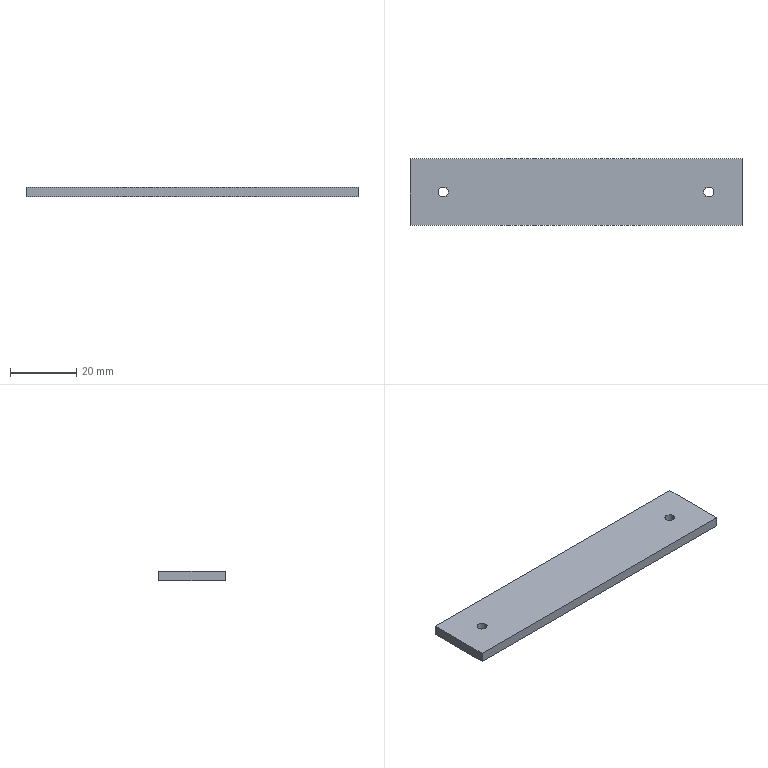Part | SolidWorks | features BaseBody 1 | 1 solid | 10 faces | box 100 x 20 x 3 mm | volume 5958 mm3 | plane 6 | cylinder 4 | commonest cylinder face diameters 3 x4
STEP:
#1=CARTESIAN_POINT('',(38.5,0.,0.));
#2=VERTEX_POINT('',#1);
#3=CARTESIAN_POINT('',(41.5,0.,0.));
#4=VERTEX_POINT('',#3);
#5=CARTESIAN_POINT('',(40.,0.,0.));
#6=DIRECTION('',(0.,0.,1.));
#7=DIRECTION('',(1.,0.,0.));
#8=AXIS2_PLACEMENT_3D('',#5,#6,#7);
#9=CIRCLE('',#8,1.5);
#10=EDGE_CURVE('',#2,#4,#9,.T.);
#11=ORIENTED_EDGE('',*,*,#10,.F.);
#12=CARTESIAN_POINT('',(38.5,0.,3.));
#13=VERTEX_POINT('',#12);
#14=CARTESIAN_POINT('',(38.5,0.,0.));
#15=DIRECTION('',(0.,0.,1.));
#16=VECTOR('',#15,1000.);
#17=LINE('',#14,#16);
#18=EDGE_CURVE('',#2,#13,#17,.T.);
#19=ORIENTED_EDGE('',*,*,#18,.T.);
#20=CARTESIAN_POINT('',(41.5,0.,3.));
#21=VERTEX_POINT('',#20);
#22=CARTESIAN_POINT('',(40.,0.,3.));
#23=DIRECTION('',(0.,0.,-1.));
#24=DIRECTION('',(1.,0.,0.));
#25=AXIS2_PLACEMENT_3D('',#22,#23,#24);
#26=CIRCLE('',#25,1.5);
#27=EDGE_CURVE('',#21,#13,#26,.T.);
#28=ORIENTED_EDGE('',*,*,#27,.F.);
#29=CARTESIAN_POINT('',(41.5,0.,0.));
#30=DIRECTION('',(0.,0.,1.));
#31=VECTOR('',#30,1000.);
#32=LINE('',#29,#31);
#33=EDGE_CURVE('',#4,#21,#32,.T.);
#34=ORIENTED_EDGE('',*,*,#33,.F.);
#35=EDGE_LOOP('',(#11,#19,#28,#34));
#36=FACE_OUTER_BOUND('',#35,.T.);
#37=CARTESIAN_POINT('',(40.,0.,0.));
#38=DIRECTION('',(0.,0.,1.));
#39=DIRECTION('',(1.,0.,0.));
#40=AXIS2_PLACEMENT_3D('',#37,#38,#39);
#41=CYLINDRICAL_SURFACE('',#40,1.5);
#42=ADVANCED_FACE('',(#36),#41,.F.);
#43=CARTESIAN_POINT('',(-41.5,0.,0.));
#44=VERTEX_POINT('',#43);
#45=CARTESIAN_POINT('',(-38.5,0.,0.));
#46=VERTEX_POINT('',#45);
#47=CARTESIAN_POINT('',(-40.,0.,0.));
#48=DIRECTION('',(0.,0.,1.));
#49=DIRECTION('',(1.,0.,0.));
#50=AXIS2_PLACEMENT_3D('',#47,#48,#49);
#51=CIRCLE('',#50,1.5);
#52=EDGE_CURVE('',#44,#46,#51,.T.);
#53=ORIENTED_EDGE('',*,*,#52,.F.);
#54=CARTESIAN_POINT('',(-41.5,0.,3.));
#55=VERTEX_POINT('',#54);
#56=CARTESIAN_POINT('',(-41.5,0.,0.));
#57=DIRECTION('',(0.,0.,1.));
#58=VECTOR('',#57,1000.);
#59=LINE('',#56,#58);
#60=EDGE_CURVE('',#44,#55,#59,.T.);
#61=ORIENTED_EDGE('',*,*,#60,.T.);
#62=CARTESIAN_POINT('',(-38.5,0.,3.));
#63=VERTEX_POINT('',#62);
#64=CARTESIAN_POINT('',(-40.,0.,3.));
#65=DIRECTION('',(0.,0.,-1.));
#66=DIRECTION('',(1.,0.,0.));
#67=AXIS2_PLACEMENT_3D('',#64,#65,#66);
#68=CIRCLE('',#67,1.5);
#69=EDGE_CURVE('',#63,#55,#68,.T.);
#70=ORIENTED_EDGE('',*,*,#69,.F.);
#71=CARTESIAN_POINT('',(-38.5,0.,0.));
#72=DIRECTION('',(0.,0.,1.));
#73=VECTOR('',#72,1000.);
#74=LINE('',#71,#73);
#75=EDGE_CURVE('',#46,#63,#74,.T.);
#76=ORIENTED_EDGE('',*,*,#75,.F.);
#77=EDGE_LOOP('',(#53,#61,#70,#76));
#78=FACE_OUTER_BOUND('',#77,.T.);
#79=CARTESIAN_POINT('',(-40.,0.,0.));
#80=DIRECTION('',(0.,0.,1.));
#81=DIRECTION('',(1.,0.,0.));
#82=AXIS2_PLACEMENT_3D('',#79,#80,#81);
#83=CYLINDRICAL_SURFACE('',#82,1.5);
#84=ADVANCED_FACE('',(#78),#83,.F.);
#85=CARTESIAN_POINT('',(-50.,10.,3.));
#86=VERTEX_POINT('',#85);
#87=CARTESIAN_POINT('',(-50.,-10.,3.));
#88=VERTEX_POINT('',#87);
#89=CARTESIAN_POINT('',(-50.,0.,3.));
#90=DIRECTION('',(0.,-1.,0.));
#91=VECTOR('',#90,1000.);
#92=LINE('',#89,#91);
#93=EDGE_CURVE('',#86,#88,#92,.T.);
#94=ORIENTED_EDGE('',*,*,#93,.T.);
#95=CARTESIAN_POINT('',(50.,-10.,3.));
#96=VERTEX_POINT('',#95);
#97=CARTESIAN_POINT('',(0.,-10.,3.));
#98=DIRECTION('',(1.,0.,0.));
#99=VECTOR('',#98,1000.);
#100=LINE('',#97,#99);
#101=EDGE_CURVE('',#88,#96,#100,.T.);
#102=ORIENTED_EDGE('',*,*,#101,.T.);
#103=CARTESIAN_POINT('',(50.,10.,3.));
#104=VERTEX_POINT('',#103);
#105=CARTESIAN_POINT('',(50.,0.,3.));
#106=DIRECTION('',(0.,1.,0.));
#107=VECTOR('',#106,1000.);
#108=LINE('',#105,#107);
#109=EDGE_CURVE('',#96,#104,#108,.T.);
#110=ORIENTED_EDGE('',*,*,#109,.T.);
#111=CARTESIAN_POINT('',(0.,10.,3.));
#112=DIRECTION('',(-1.,0.,0.));
#113=VECTOR('',#112,1000.);
#114=LINE('',#111,#113);
#115=EDGE_CURVE('',#104,#86,#114,.T.);
#116=ORIENTED_EDGE('',*,*,#115,.T.);
#117=EDGE_LOOP('',(#94,#102,#110,#116));
#118=FACE_OUTER_BOUND('',#117,.T.);
#119=ORIENTED_EDGE('',*,*,#27,.T.);
#120=CARTESIAN_POINT('',(40.,0.,3.));
#121=DIRECTION('',(0.,0.,-1.));
#122=DIRECTION('',(1.,0.,0.));
#123=AXIS2_PLACEMENT_3D('',#120,#121,#122);
#124=CIRCLE('',#123,1.5);
#125=EDGE_CURVE('',#13,#21,#124,.T.);
#126=ORIENTED_EDGE('',*,*,#125,.T.);
#127=EDGE_LOOP('',(#119,#126));
#128=FACE_BOUND('',#127,.T.);
#129=ORIENTED_EDGE('',*,*,#69,.T.);
#130=CARTESIAN_POINT('',(-40.,0.,3.));
#131=DIRECTION('',(0.,0.,-1.));
#132=DIRECTION('',(1.,0.,0.));
#133=AXIS2_PLACEMENT_3D('',#130,#131,#132);
#134=CIRCLE('',#133,1.5);
#135=EDGE_CURVE('',#55,#63,#134,.T.);
#136=ORIENTED_EDGE('',*,*,#135,.T.);
#137=EDGE_LOOP('',(#129,#136));
#138=FACE_BOUND('',#137,.T.);
#139=CARTESIAN_POINT('',(0.,0.,3.));
#140=DIRECTION('',(0.,0.,1.));
#141=DIRECTION('',(1.,0.,0.));
#142=AXIS2_PLACEMENT_3D('',#139,#140,#141);
#143=PLANE('',#142);
#144=ADVANCED_FACE('',(#118,#128,#138),#143,.T.);
#145=CARTESIAN_POINT('',(50.,-10.,0.));
#146=VERTEX_POINT('',#145);
#147=CARTESIAN_POINT('',(50.,-10.,3.));
#148=DIRECTION('',(0.,0.,-1.));
#149=VECTOR('',#148,1000.);
#150=LINE('',#147,#149);
#151=EDGE_CURVE('',#96,#146,#150,.T.);
#152=ORIENTED_EDGE('',*,*,#151,.F.);
#153=ORIENTED_EDGE('',*,*,#101,.F.);
#154=CARTESIAN_POINT('',(-50.,-10.,0.));
#155=VERTEX_POINT('',#154);
#156=CARTESIAN_POINT('',(-50.,-10.,3.));
#157=DIRECTION('',(0.,0.,1.));
#158=VECTOR('',#157,1000.);
#159=LINE('',#156,#158);
#160=EDGE_CURVE('',#155,#88,#159,.T.);
#161=ORIENTED_EDGE('',*,*,#160,.F.);
#162=CARTESIAN_POINT('',(-50.,-10.,0.));
#163=DIRECTION('',(-1.,0.,0.));
#164=VECTOR('',#163,1000.);
#165=LINE('',#162,#164);
#166=EDGE_CURVE('',#146,#155,#165,.T.);
#167=ORIENTED_EDGE('',*,*,#166,.F.);
#168=EDGE_LOOP('',(#152,#153,#161,#167));
#169=FACE_OUTER_BOUND('',#168,.T.);
#170=CARTESIAN_POINT('',(-50.,-10.,3.));
#171=DIRECTION('',(0.,1.,0.));
#172=DIRECTION('',(0.,0.,1.));
#173=AXIS2_PLACEMENT_3D('',#170,#171,#172);
#174=PLANE('',#173);
#175=ADVANCED_FACE('',(#169),#174,.F.);
#176=ORIENTED_EDGE('',*,*,#160,.T.);
#177=ORIENTED_EDGE('',*,*,#93,.F.);
#178=CARTESIAN_POINT('',(-50.,10.,0.));
#179=VERTEX_POINT('',#178);
#180=CARTESIAN_POINT('',(-50.,10.,3.));
#181=DIRECTION('',(0.,0.,1.));
#182=VECTOR('',#181,1000.);
#183=LINE('',#180,#182);
#184=EDGE_CURVE('',#179,#86,#183,.T.);
#185=ORIENTED_EDGE('',*,*,#184,.F.);
#186=CARTESIAN_POINT('',(-50.,10.,0.));
#187=DIRECTION('',(0.,1.,0.));
#188=VECTOR('',#187,1000.);
#189=LINE('',#186,#188);
#190=EDGE_CURVE('',#155,#179,#189,.T.);
#191=ORIENTED_EDGE('',*,*,#190,.F.);
#192=EDGE_LOOP('',(#176,#177,#185,#191));
#193=FACE_OUTER_BOUND('',#192,.T.);
#194=CARTESIAN_POINT('',(-50.,10.,3.));
#195=DIRECTION('',(1.,0.,0.));
#196=DIRECTION('',(0.,0.,-1.));
#197=AXIS2_PLACEMENT_3D('',#194,#195,#196);
#198=PLANE('',#197);
#199=ADVANCED_FACE('',(#193),#198,.F.);
#200=ORIENTED_EDGE('',*,*,#184,.T.);
#201=ORIENTED_EDGE('',*,*,#115,.F.);
#202=CARTESIAN_POINT('',(50.,10.,0.));
#203=VERTEX_POINT('',#202);
#204=CARTESIAN_POINT('',(50.,10.,3.));
#205=DIRECTION('',(0.,0.,1.));
#206=VECTOR('',#205,1000.);
#207=LINE('',#204,#206);
#208=EDGE_CURVE('',#203,#104,#207,.T.);
#209=ORIENTED_EDGE('',*,*,#208,.F.);
#210=CARTESIAN_POINT('',(-50.,10.,0.));
#211=DIRECTION('',(1.,0.,0.));
#212=VECTOR('',#211,1000.);
#213=LINE('',#210,#212);
#214=EDGE_CURVE('',#179,#203,#213,.T.);
#215=ORIENTED_EDGE('',*,*,#214,.F.);
#216=EDGE_LOOP('',(#200,#201,#209,#215));
#217=FACE_OUTER_BOUND('',#216,.T.);
#218=CARTESIAN_POINT('',(-50.,10.,3.));
#219=DIRECTION('',(0.,-1.,0.));
#220=DIRECTION('',(0.,0.,-1.));
#221=AXIS2_PLACEMENT_3D('',#218,#219,#220);
#222=PLANE('',#221);
#223=ADVANCED_FACE('',(#217),#222,.F.);
#224=ORIENTED_EDGE('',*,*,#208,.T.);
#225=ORIENTED_EDGE('',*,*,#109,.F.);
#226=ORIENTED_EDGE('',*,*,#151,.T.);
#227=CARTESIAN_POINT('',(50.,10.,0.));
#228=DIRECTION('',(0.,-1.,0.));
#229=VECTOR('',#228,1000.);
#230=LINE('',#227,#229);
#231=EDGE_CURVE('',#203,#146,#230,.T.);
#232=ORIENTED_EDGE('',*,*,#231,.F.);
#233=EDGE_LOOP('',(#224,#225,#226,#232));
#234=FACE_OUTER_BOUND('',#233,.T.);
#235=CARTESIAN_POINT('',(50.,10.,3.));
#236=DIRECTION('',(-1.,0.,0.));
#237=DIRECTION('',(0.,0.,1.));
#238=AXIS2_PLACEMENT_3D('',#235,#236,#237);
#239=PLANE('',#238);
#240=ADVANCED_FACE('',(#234),#239,.F.);
#241=ORIENTED_EDGE('',*,*,#18,.F.);
#242=CARTESIAN_POINT('',(40.,0.,0.));
#243=DIRECTION('',(0.,0.,1.));
#244=DIRECTION('',(1.,0.,0.));
#245=AXIS2_PLACEMENT_3D('',#242,#243,#244);
#246=CIRCLE('',#245,1.5);
#247=EDGE_CURVE('',#4,#2,#246,.T.);
#248=ORIENTED_EDGE('',*,*,#247,.F.);
#249=ORIENTED_EDGE('',*,*,#33,.T.);
#250=ORIENTED_EDGE('',*,*,#125,.F.);
#251=EDGE_LOOP('',(#241,#248,#249,#250));
#252=FACE_OUTER_BOUND('',#251,.T.);
#253=CARTESIAN_POINT('',(40.,0.,0.));
#254=DIRECTION('',(0.,0.,1.));
#255=DIRECTION('',(1.,0.,0.));
#256=AXIS2_PLACEMENT_3D('',#253,#254,#255);
#257=CYLINDRICAL_SURFACE('',#256,1.5);
#258=ADVANCED_FACE('',(#252),#257,.F.);
#259=ORIENTED_EDGE('',*,*,#60,.F.);
#260=CARTESIAN_POINT('',(-40.,0.,0.));
#261=DIRECTION('',(0.,0.,1.));
#262=DIRECTION('',(1.,0.,0.));
#263=AXIS2_PLACEMENT_3D('',#260,#261,#262);
#264=CIRCLE('',#263,1.5);
#265=EDGE_CURVE('',#46,#44,#264,.T.);
#266=ORIENTED_EDGE('',*,*,#265,.F.);
#267=ORIENTED_EDGE('',*,*,#75,.T.);
#268=ORIENTED_EDGE('',*,*,#135,.F.);
#269=EDGE_LOOP('',(#259,#266,#267,#268));
#270=FACE_OUTER_BOUND('',#269,.T.);
#271=CARTESIAN_POINT('',(-40.,0.,0.));
#272=DIRECTION('',(0.,0.,1.));
#273=DIRECTION('',(1.,0.,0.));
#274=AXIS2_PLACEMENT_3D('',#271,#272,#273);
#275=CYLINDRICAL_SURFACE('',#274,1.5);
#276=ADVANCED_FACE('',(#270),#275,.F.);
#277=ORIENTED_EDGE('',*,*,#166,.T.);
#278=ORIENTED_EDGE('',*,*,#190,.T.);
#279=ORIENTED_EDGE('',*,*,#214,.T.);
#280=ORIENTED_EDGE('',*,*,#231,.T.);
#281=EDGE_LOOP('',(#277,#278,#279,#280));
#282=FACE_OUTER_BOUND('',#281,.T.);
#283=ORIENTED_EDGE('',*,*,#247,.T.);
#284=ORIENTED_EDGE('',*,*,#10,.T.);
#285=EDGE_LOOP('',(#283,#284));
#286=FACE_BOUND('',#285,.T.);
#287=ORIENTED_EDGE('',*,*,#265,.T.);
#288=ORIENTED_EDGE('',*,*,#52,.T.);
#289=EDGE_LOOP('',(#287,#288));
#290=FACE_BOUND('',#289,.T.);
#291=CARTESIAN_POINT('',(0.,0.,0.));
#292=DIRECTION('',(0.,0.,1.));
#293=DIRECTION('',(1.,0.,0.));
#294=AXIS2_PLACEMENT_3D('',#291,#292,#293);
#295=PLANE('',#294);
#296=ADVANCED_FACE('',(#282,#286,#290),#295,.F.);
#297=CLOSED_SHELL('',(#42,#84,#144,#175,#199,#223,#240,#258,#276,#296));
#298=MANIFOLD_SOLID_BREP('',#297);
#299=CARTESIAN_POINT('',(0.,0.,0.));
#300=DIRECTION('',(0.,0.,1.));
#301=DIRECTION('',(1.,0.,0.));
#302=AXIS2_PLACEMENT_3D('',#299,#300,#301);
#303=(LENGTH_UNIT()NAMED_UNIT(*)SI_UNIT(.MILLI.,.METRE.));
#304=UNCERTAINTY_MEASURE_WITH_UNIT(LENGTH_MEASURE(0.00001),#303,'','');
#305=(NAMED_UNIT(*)PLANE_ANGLE_UNIT()SI_UNIT($,.RADIAN.));
#306=(NAMED_UNIT(*)SI_UNIT($,.STERADIAN.)SOLID_ANGLE_UNIT());
#307=(GEOMETRIC_REPRESENTATION_CONTEXT(3)GLOBAL_UNCERTAINTY_ASSIGNED_CONTEXT((#304))GLOBAL_UNIT_ASSIGNED_CONTEXT((#303,#305,#306))REPRESENTATION_CONTEXT('',''));
#308=ADVANCED_BREP_SHAPE_REPRESENTATION('',(#298,#302),#307);